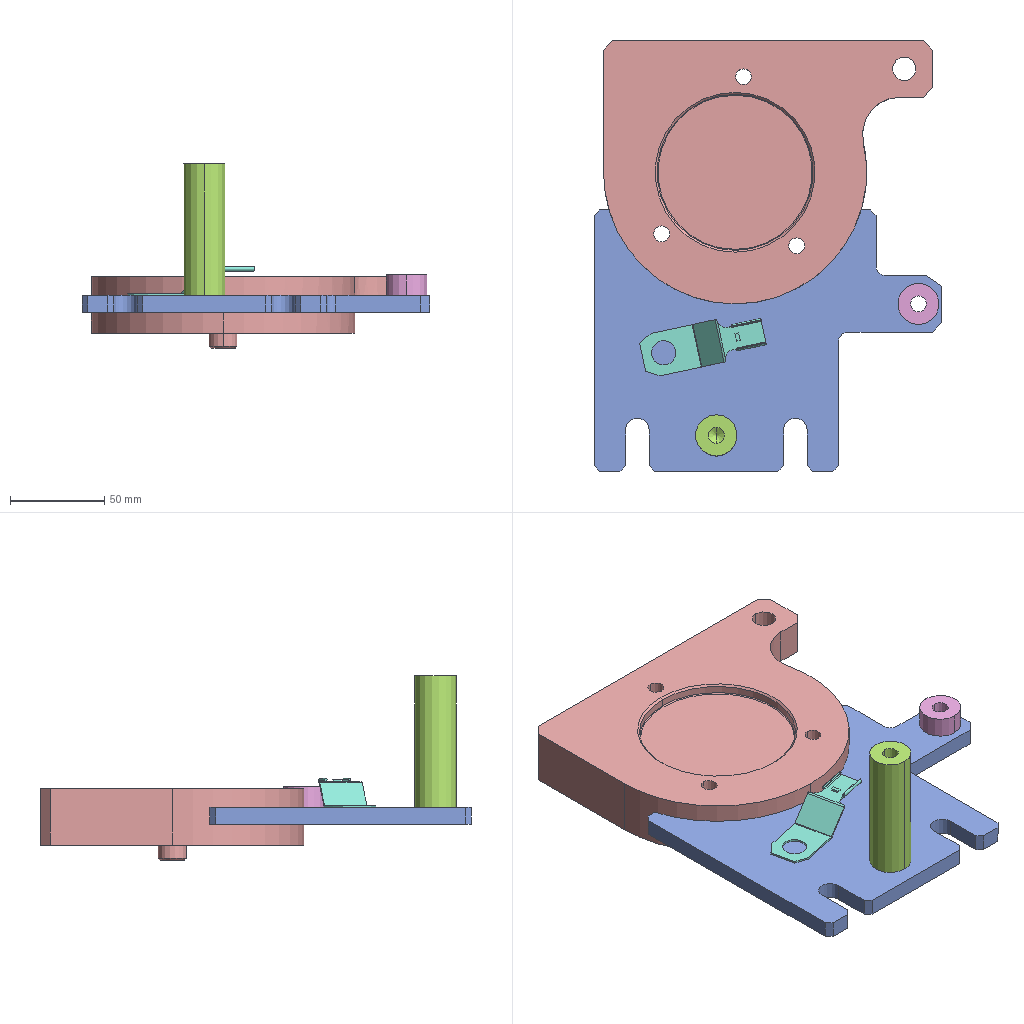Assembly | SolidWorks | 5 different items | 5 placed | box 185 x 229 x 98 mm
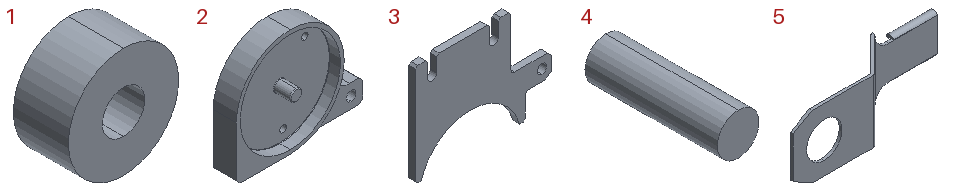Parts list (item | quantity | size | volume | features):
1 | x1 | 22 x 11 x 22 mm | 3557 mm3 | features Extrusion 1, HoleWzd 1
2 | x1 | 175 x 38 x 140 mm | 313299 mm3 | features ICE 5, HoleWzd 2, Chamfer 1, Fillet 1, FlatPattern 1, SMBaseFlange 1, SheetMetal 1
3 | x1 | 185 x 9 x 139 mm | 131664 mm3 | features FlatPattern 1, SMBaseFlange 1, SheetMetal 1
4 | x1 | 22 x 70 x 22 mm | 25142 mm3 | features Extrusion 1, HoleWzd 1
5 | x1 | 65.7 x 15.573 x 23.06 mm | 1342 mm3 | features BaseBody 1
Mates (type | each side: item.copy, entity, surface, feature):
Concentric | 2.1 face cylinder Base-Flange1 | 3.1 face cylinder Base-Flange1
DistanceDim | 3.1 face plane Base-Flange1 | 2.1 face plane Base-Flange1
Parallel | 2.1 plane | 3.1 plane
Coincident | 3.1 face plane Base-Flange1 | 4.1 face plane Boss-Extrude1
DistanceDim | 4.1 plane | 2.1 face plane Base-Flange1
DistanceDim | 4.1 plane | 2.1 face cylinder Cut-Extrude2
Coincident | 3.1 face plane Base-Flange1 | 1.1 face plane Boss-Extrude1
Concentric | 3.1 face cylinder Base-Flange1 | 1.1 face cylinder M10 Tapped Hole1
Parallel | 3.1 face plane Base-Flange1 | 1.1 plane
Coincident | 3.1 face plane Base-Flange1 | 5.1 face plane Imported1
PlanarAngleDim | 5.1 face plane Imported1 | 3.1 face plane Base-Flange1
DistanceDim | 5.1 face cylinder Imported1 | 1.1 plane | 2 times